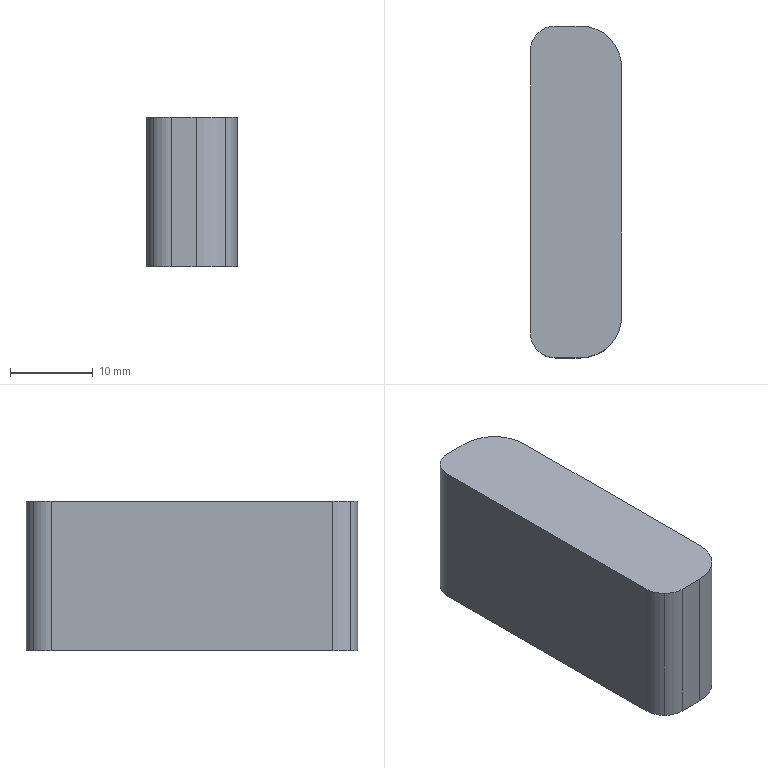Part | STEP file | ASND-0110-6.3aq | 1 solid | 14 faces | box 11 x 40 x 18 mm | volume 7657 mm3 | cylinder 8 | plane 6 | commonest cylinder face diameters 6 x4 10 x4
STEP:
#1=CARTESIAN_POINT('',(0.,0.,0.));
#2=DIRECTION('',(0.,0.,1.));
#3=DIRECTION('',(1.,0.,0.));
#4=AXIS2_PLACEMENT_3D('',#1,#2,#3);
#5=CARTESIAN_POINT('',(-191.546,183.474,-18.));
#6=VERTEX_POINT('',#5);
#7=CARTESIAN_POINT('',(-193.011,187.009,-18.));
#8=VERTEX_POINT('',#7);
#9=CARTESIAN_POINT('',(-196.546,183.474,-18.));
#10=DIRECTION('',(0.,0.,1.));
#11=DIRECTION('',(0.7071,0.7071,0.));
#12=AXIS2_PLACEMENT_3D('',#9,#10,#11);
#13=CIRCLE('',#12,5.);
#14=CARTESIAN_POINT('',(-196.546,183.474,-18.));
#15=DIRECTION('',(0.,0.,1.));
#16=DIRECTION('',(0.7071,0.7071,0.));
#17=AXIS2_PLACEMENT_3D('',#14,#15,#16);
#18=CYLINDRICAL_SURFACE('',#17,5.);
#19=CARTESIAN_POINT('',(0.,0.));
#20=DIRECTION('',(1.,0.));
#21=VECTOR('',#20,1.);
#22=LINE('',#19,#21);
#23=(GEOMETRIC_REPRESENTATION_CONTEXT(2)PARAMETRIC_REPRESENTATION_CONTEXT()REPRESENTATION_CONTEXT('',''));
#24=DEFINITIONAL_REPRESENTATION('',(#22),#23);
#25=PCURVE('',#18,#24);
#26=CARTESIAN_POINT('',(-195.546,183.474,-18.));
#27=DIRECTION('',(0.,0.,1.));
#28=DIRECTION('',(0.7071,0.7071,0.));
#29=AXIS2_PLACEMENT_3D('',#26,#27,#28);
#30=PLANE('',#29);
#31=CARTESIAN_POINT('',(-0.7071,0.7071));
#32=DIRECTION('',(1.,0.));
#33=AXIS2_PLACEMENT_2D('',#31,#32);
#34=CIRCLE('',#33,5.);
#35=(GEOMETRIC_REPRESENTATION_CONTEXT(2)PARAMETRIC_REPRESENTATION_CONTEXT()REPRESENTATION_CONTEXT('',''));
#36=DEFINITIONAL_REPRESENTATION('',(#34),#35);
#37=PCURVE('',#30,#36);
#38=SURFACE_CURVE('',#13,(#25,#37),.PCURVE_S1.);
#39=EDGE_CURVE('',#6,#8,#38,.T.);
#40=ORIENTED_EDGE('',*,*,#39,.T.);
#41=CARTESIAN_POINT('',(-193.011,187.009,0.));
#42=VERTEX_POINT('',#41);
#43=CARTESIAN_POINT('',(-193.011,187.009,-18.));
#44=DIRECTION('',(0.,0.,1.));
#45=VECTOR('',#44,1.);
#46=LINE('',#43,#45);
#47=CARTESIAN_POINT('',(6.283,0.));
#48=DIRECTION('',(0.,1.));
#49=VECTOR('',#48,1.);
#50=LINE('',#47,#49);
#51=(GEOMETRIC_REPRESENTATION_CONTEXT(2)PARAMETRIC_REPRESENTATION_CONTEXT()REPRESENTATION_CONTEXT('',''));
#52=DEFINITIONAL_REPRESENTATION('',(#50),#51);
#53=PCURVE('',#18,#52);
#54=CARTESIAN_POINT('',(-196.546,183.474,-18.));
#55=DIRECTION('',(0.,0.,1.));
#56=DIRECTION('',(0.7071,0.7071,0.));
#57=AXIS2_PLACEMENT_3D('',#54,#55,#56);
#58=CYLINDRICAL_SURFACE('',#57,5.);
#59=CARTESIAN_POINT('',(0.,0.));
#60=DIRECTION('',(0.,1.));
#61=VECTOR('',#60,1.);
#62=LINE('',#59,#61);
#63=(GEOMETRIC_REPRESENTATION_CONTEXT(2)PARAMETRIC_REPRESENTATION_CONTEXT()REPRESENTATION_CONTEXT('',''));
#64=DEFINITIONAL_REPRESENTATION('',(#62),#63);
#65=PCURVE('',#58,#64);
#66=SURFACE_CURVE('',#46,(#53,#65),.PCURVE_S1.);
#67=EDGE_CURVE('',#8,#42,#66,.T.);
#68=ORIENTED_EDGE('',*,*,#67,.T.);
#69=CARTESIAN_POINT('',(-191.546,183.474,0.));
#70=VERTEX_POINT('',#69);
#71=CARTESIAN_POINT('',(-196.546,183.474,0.));
#72=DIRECTION('',(0.,0.,-1.));
#73=DIRECTION('',(0.7071,0.7071,0.));
#74=AXIS2_PLACEMENT_3D('',#71,#72,#73);
#75=CIRCLE('',#74,5.);
#76=CARTESIAN_POINT('',(6.283,18.));
#77=DIRECTION('',(-1.,0.));
#78=VECTOR('',#77,1.);
#79=LINE('',#76,#78);
#80=(GEOMETRIC_REPRESENTATION_CONTEXT(2)PARAMETRIC_REPRESENTATION_CONTEXT()REPRESENTATION_CONTEXT('',''));
#81=DEFINITIONAL_REPRESENTATION('',(#79),#80);
#82=PCURVE('',#18,#81);
#83=CARTESIAN_POINT('',(-195.546,183.474,0.));
#84=DIRECTION('',(0.,0.,1.));
#85=DIRECTION('',(0.7071,0.7071,0.));
#86=AXIS2_PLACEMENT_3D('',#83,#84,#85);
#87=PLANE('',#86);
#88=CARTESIAN_POINT('',(4.293,0.7071));
#89=CARTESIAN_POINT('',(4.293,-7.953));
#90=CARTESIAN_POINT('',(-3.207,-3.623));
#91=CARTESIAN_POINT('',(-10.707,0.7071));
#92=CARTESIAN_POINT('',(-3.207,5.037));
#93=CARTESIAN_POINT('',(4.293,9.367));
#94=CARTESIAN_POINT('',(4.293,0.7071));
#95=(BOUNDED_CURVE()B_SPLINE_CURVE(2,(#88,#89,#90,#91,#92,#93,#94),.UNSPECIFIED.,.T.,.F.)B_SPLINE_CURVE_WITH_KNOTS((1,2,2,2,2,1),(-2.094,0.,2.094,4.189,6.283,8.378),.UNSPECIFIED.)CURVE()GEOMETRIC_REPRESENTATION_ITEM()RATIONAL_B_SPLINE_CURVE((1.,0.5,1.,0.5,1.,0.5,1.))REPRESENTATION_ITEM(''));
#96=(GEOMETRIC_REPRESENTATION_CONTEXT(2)PARAMETRIC_REPRESENTATION_CONTEXT()REPRESENTATION_CONTEXT('',''));
#97=DEFINITIONAL_REPRESENTATION('',(#95),#96);
#98=PCURVE('',#87,#97);
#99=SURFACE_CURVE('',#75,(#82,#98),.PCURVE_S1.);
#100=EDGE_CURVE('',#42,#70,#99,.T.);
#101=ORIENTED_EDGE('',*,*,#100,.T.);
#102=CARTESIAN_POINT('',(-191.546,183.474,-18.));
#103=DIRECTION('',(0.,0.,-1.));
#104=VECTOR('',#103,1.);
#105=LINE('',#102,#104);
#106=CARTESIAN_POINT('',(5.498,0.));
#107=DIRECTION('',(0.,-1.));
#108=VECTOR('',#107,1.);
#109=LINE('',#106,#108);
#110=(GEOMETRIC_REPRESENTATION_CONTEXT(2)PARAMETRIC_REPRESENTATION_CONTEXT()REPRESENTATION_CONTEXT('',''));
#111=DEFINITIONAL_REPRESENTATION('',(#109),#110);
#112=PCURVE('',#18,#111);
#113=CARTESIAN_POINT('',(-191.546,183.474,-18.));
#114=DIRECTION('',(1.,0.,0.));
#115=DIRECTION('',(0.,0.7071,0.7071));
#116=AXIS2_PLACEMENT_3D('',#113,#114,#115);
#117=PLANE('',#116);
#118=CARTESIAN_POINT('',(0.,0.));
#119=DIRECTION('',(-0.7071,-0.7071));
#120=VECTOR('',#119,1.);
#121=LINE('',#118,#120);
#122=(GEOMETRIC_REPRESENTATION_CONTEXT(2)PARAMETRIC_REPRESENTATION_CONTEXT()REPRESENTATION_CONTEXT('',''));
#123=DEFINITIONAL_REPRESENTATION('',(#121),#122);
#124=PCURVE('',#117,#123);
#125=SURFACE_CURVE('',#105,(#112,#124),.PCURVE_S1.);
#126=EDGE_CURVE('',#70,#6,#125,.T.);
#127=ORIENTED_EDGE('',*,*,#126,.T.);
#128=EDGE_LOOP('',(#40,#68,#101,#127));
#129=FACE_BOUND('',#128,.T.);
#130=ADVANCED_FACE('',(#129),#18,.T.);
#131=CARTESIAN_POINT('',(-196.546,148.474,-18.));
#132=VERTEX_POINT('',#131);
#133=CARTESIAN_POINT('',(-193.011,149.938,-18.));
#134=VERTEX_POINT('',#133);
#135=CARTESIAN_POINT('',(-196.546,153.474,-18.));
#136=DIRECTION('',(0.,0.,1.));
#137=DIRECTION('',(0.7071,-0.7071,0.));
#138=AXIS2_PLACEMENT_3D('',#135,#136,#137);
#139=CIRCLE('',#138,5.);
#140=CARTESIAN_POINT('',(-196.546,153.474,-18.));
#141=DIRECTION('',(0.,0.,1.));
#142=DIRECTION('',(0.7071,-0.7071,0.));
#143=AXIS2_PLACEMENT_3D('',#140,#141,#142);
#144=CYLINDRICAL_SURFACE('',#143,5.);
#145=CARTESIAN_POINT('',(0.,0.));
#146=DIRECTION('',(1.,0.));
#147=VECTOR('',#146,1.);
#148=LINE('',#145,#147);
#149=(GEOMETRIC_REPRESENTATION_CONTEXT(2)PARAMETRIC_REPRESENTATION_CONTEXT()REPRESENTATION_CONTEXT('',''));
#150=DEFINITIONAL_REPRESENTATION('',(#148),#149);
#151=PCURVE('',#144,#150);
#152=CARTESIAN_POINT('',(-21.92,-20.506));
#153=DIRECTION('',(0.,-1.));
#154=AXIS2_PLACEMENT_2D('',#152,#153);
#155=CIRCLE('',#154,5.);
#156=(GEOMETRIC_REPRESENTATION_CONTEXT(2)PARAMETRIC_REPRESENTATION_CONTEXT()REPRESENTATION_CONTEXT('',''));
#157=DEFINITIONAL_REPRESENTATION('',(#155),#156);
#158=PCURVE('',#30,#157);
#159=SURFACE_CURVE('',#139,(#151,#158),.PCURVE_S1.);
#160=EDGE_CURVE('',#132,#134,#159,.T.);
#161=ORIENTED_EDGE('',*,*,#160,.T.);
#162=CARTESIAN_POINT('',(-193.011,149.938,0.));
#163=VERTEX_POINT('',#162);
#164=CARTESIAN_POINT('',(-193.011,149.938,-18.));
#165=DIRECTION('',(0.,0.,1.));
#166=VECTOR('',#165,1.);
#167=LINE('',#164,#166);
#168=CARTESIAN_POINT('',(6.283,0.));
#169=DIRECTION('',(0.,1.));
#170=VECTOR('',#169,1.);
#171=LINE('',#168,#170);
#172=(GEOMETRIC_REPRESENTATION_CONTEXT(2)PARAMETRIC_REPRESENTATION_CONTEXT()REPRESENTATION_CONTEXT('',''));
#173=DEFINITIONAL_REPRESENTATION('',(#171),#172);
#174=PCURVE('',#144,#173);
#175=CARTESIAN_POINT('',(-196.546,153.474,-18.));
#176=DIRECTION('',(0.,0.,1.));
#177=DIRECTION('',(0.7071,-0.7071,0.));
#178=AXIS2_PLACEMENT_3D('',#175,#176,#177);
#179=CYLINDRICAL_SURFACE('',#178,5.);
#180=CARTESIAN_POINT('',(0.,0.));
#181=DIRECTION('',(0.,1.));
#182=VECTOR('',#181,1.);
#183=LINE('',#180,#182);
#184=(GEOMETRIC_REPRESENTATION_CONTEXT(2)PARAMETRIC_REPRESENTATION_CONTEXT()REPRESENTATION_CONTEXT('',''));
#185=DEFINITIONAL_REPRESENTATION('',(#183),#184);
#186=PCURVE('',#179,#185);
#187=SURFACE_CURVE('',#167,(#174,#186),.PCURVE_S1.);
#188=EDGE_CURVE('',#134,#163,#187,.T.);
#189=ORIENTED_EDGE('',*,*,#188,.T.);
#190=CARTESIAN_POINT('',(-196.546,148.474,0.));
#191=VERTEX_POINT('',#190);
#192=CARTESIAN_POINT('',(-196.546,153.474,0.));
#193=DIRECTION('',(0.,0.,-1.));
#194=DIRECTION('',(0.7071,-0.7071,0.));
#195=AXIS2_PLACEMENT_3D('',#192,#193,#194);
#196=CIRCLE('',#195,5.);
#197=CARTESIAN_POINT('',(6.283,18.));
#198=DIRECTION('',(-1.,0.));
#199=VECTOR('',#198,1.);
#200=LINE('',#197,#199);
#201=(GEOMETRIC_REPRESENTATION_CONTEXT(2)PARAMETRIC_REPRESENTATION_CONTEXT()REPRESENTATION_CONTEXT('',''));
#202=DEFINITIONAL_REPRESENTATION('',(#200),#201);
#203=PCURVE('',#144,#202);
#204=CARTESIAN_POINT('',(-21.92,-25.506));
#205=CARTESIAN_POINT('',(-30.581,-25.506));
#206=CARTESIAN_POINT('',(-26.25,-18.006));
#207=CARTESIAN_POINT('',(-21.92,-10.506));
#208=CARTESIAN_POINT('',(-17.59,-18.006));
#209=CARTESIAN_POINT('',(-13.26,-25.506));
#210=CARTESIAN_POINT('',(-21.92,-25.506));
#211=(BOUNDED_CURVE()B_SPLINE_CURVE(2,(#204,#205,#206,#207,#208,#209,#210),.UNSPECIFIED.,.T.,.F.)B_SPLINE_CURVE_WITH_KNOTS((1,2,2,2,2,1),(-2.094,0.,2.094,4.189,6.283,8.378),.UNSPECIFIED.)CURVE()GEOMETRIC_REPRESENTATION_ITEM()RATIONAL_B_SPLINE_CURVE((1.,0.5,1.,0.5,1.,0.5,1.))REPRESENTATION_ITEM(''));
#212=(GEOMETRIC_REPRESENTATION_CONTEXT(2)PARAMETRIC_REPRESENTATION_CONTEXT()REPRESENTATION_CONTEXT('',''));
#213=DEFINITIONAL_REPRESENTATION('',(#211),#212);
#214=PCURVE('',#87,#213);
#215=SURFACE_CURVE('',#196,(#203,#214),.PCURVE_S1.);
#216=EDGE_CURVE('',#163,#191,#215,.T.);
#217=ORIENTED_EDGE('',*,*,#216,.T.);
#218=CARTESIAN_POINT('',(-196.546,148.474,-18.));
#219=DIRECTION('',(0.,0.,-1.));
#220=VECTOR('',#219,1.);
#221=LINE('',#218,#220);
#222=CARTESIAN_POINT('',(5.498,0.));
#223=DIRECTION('',(0.,-1.));
#224=VECTOR('',#223,1.);
#225=LINE('',#222,#224);
#226=(GEOMETRIC_REPRESENTATION_CONTEXT(2)PARAMETRIC_REPRESENTATION_CONTEXT()REPRESENTATION_CONTEXT('',''));
#227=DEFINITIONAL_REPRESENTATION('',(#225),#226);
#228=PCURVE('',#144,#227);
#229=CARTESIAN_POINT('',(-195.546,148.474,-18.));
#230=DIRECTION('',(0.,-1.,0.));
#231=DIRECTION('',(0.7071,0.,0.7071));
#232=AXIS2_PLACEMENT_3D('',#229,#230,#231);
#233=PLANE('',#232);
#234=CARTESIAN_POINT('',(-0.7071,0.7071));
#235=DIRECTION('',(-0.7071,-0.7071));
#236=VECTOR('',#235,1.);
#237=LINE('',#234,#236);
#238=(GEOMETRIC_REPRESENTATION_CONTEXT(2)PARAMETRIC_REPRESENTATION_CONTEXT()REPRESENTATION_CONTEXT('',''));
#239=DEFINITIONAL_REPRESENTATION('',(#237),#238);
#240=PCURVE('',#233,#239);
#241=SURFACE_CURVE('',#221,(#228,#240),.PCURVE_S1.);
#242=EDGE_CURVE('',#191,#132,#241,.T.);
#243=ORIENTED_EDGE('',*,*,#242,.T.);
#244=EDGE_LOOP('',(#161,#189,#217,#243));
#245=FACE_BOUND('',#244,.T.);
#246=ADVANCED_FACE('',(#245),#144,.T.);
#247=CARTESIAN_POINT('',(-199.546,148.474,0.));
#248=VERTEX_POINT('',#247);
#249=CARTESIAN_POINT('',(-201.668,149.352,0.));
#250=VERTEX_POINT('',#249);
#251=CARTESIAN_POINT('',(-199.546,151.474,0.));
#252=DIRECTION('',(0.,0.,-1.));
#253=DIRECTION('',(-0.7071,-0.7071,0.));
#254=AXIS2_PLACEMENT_3D('',#251,#252,#253);
#255=CIRCLE('',#254,3.);
#256=CARTESIAN_POINT('',(-199.546,151.474,-18.));
#257=DIRECTION('',(0.,0.,-1.));
#258=DIRECTION('',(-0.7071,-0.7071,0.));
#259=AXIS2_PLACEMENT_3D('',#256,#257,#258);
#260=CYLINDRICAL_SURFACE('',#259,3.);
#261=CARTESIAN_POINT('',(0.,-18.));
#262=DIRECTION('',(1.,0.));
#263=VECTOR('',#262,1.);
#264=LINE('',#261,#263);
#265=(GEOMETRIC_REPRESENTATION_CONTEXT(2)PARAMETRIC_REPRESENTATION_CONTEXT()REPRESENTATION_CONTEXT('',''));
#266=DEFINITIONAL_REPRESENTATION('',(#264),#265);
#267=PCURVE('',#260,#266);
#268=CARTESIAN_POINT('',(-28.456,-19.799));
#269=CARTESIAN_POINT('',(-28.456,-14.603));
#270=CARTESIAN_POINT('',(-23.956,-17.201));
#271=CARTESIAN_POINT('',(-19.456,-19.799));
#272=CARTESIAN_POINT('',(-23.956,-22.397));
#273=CARTESIAN_POINT('',(-28.456,-24.995));
#274=CARTESIAN_POINT('',(-28.456,-19.799));
#275=(BOUNDED_CURVE()B_SPLINE_CURVE(2,(#268,#269,#270,#271,#272,#273,#274),.UNSPECIFIED.,.T.,.F.)B_SPLINE_CURVE_WITH_KNOTS((1,2,2,2,2,1),(-2.094,0.,2.094,4.189,6.283,8.378),.UNSPECIFIED.)CURVE()GEOMETRIC_REPRESENTATION_ITEM()RATIONAL_B_SPLINE_CURVE((1.,0.5,1.,0.5,1.,0.5,1.))REPRESENTATION_ITEM(''));
#276=(GEOMETRIC_REPRESENTATION_CONTEXT(2)PARAMETRIC_REPRESENTATION_CONTEXT()REPRESENTATION_CONTEXT('',''));
#277=DEFINITIONAL_REPRESENTATION('',(#275),#276);
#278=PCURVE('',#87,#277);
#279=SURFACE_CURVE('',#255,(#267,#278),.PCURVE_S1.);
#280=EDGE_CURVE('',#248,#250,#279,.T.);
#281=ORIENTED_EDGE('',*,*,#280,.T.);
#282=CARTESIAN_POINT('',(-201.668,149.352,-18.));
#283=VERTEX_POINT('',#282);
#284=CARTESIAN_POINT('',(-201.668,149.352,-18.));
#285=DIRECTION('',(0.,0.,-1.));
#286=VECTOR('',#285,1.);
#287=LINE('',#284,#286);
#288=CARTESIAN_POINT('',(6.283,0.));
#289=DIRECTION('',(0.,1.));
#290=VECTOR('',#289,1.);
#291=LINE('',#288,#290);
#292=(GEOMETRIC_REPRESENTATION_CONTEXT(2)PARAMETRIC_REPRESENTATION_CONTEXT()REPRESENTATION_CONTEXT('',''));
#293=DEFINITIONAL_REPRESENTATION('',(#291),#292);
#294=PCURVE('',#260,#293);
#295=CARTESIAN_POINT('',(-199.546,151.474,-18.));
#296=DIRECTION('',(0.,0.,-1.));
#297=DIRECTION('',(-0.7071,-0.7071,0.));
#298=AXIS2_PLACEMENT_3D('',#295,#296,#297);
#299=CYLINDRICAL_SURFACE('',#298,3.);
#300=CARTESIAN_POINT('',(0.,0.));
#301=DIRECTION('',(0.,1.));
#302=VECTOR('',#301,1.);
#303=LINE('',#300,#302);
#304=(GEOMETRIC_REPRESENTATION_CONTEXT(2)PARAMETRIC_REPRESENTATION_CONTEXT()REPRESENTATION_CONTEXT('',''));
#305=DEFINITIONAL_REPRESENTATION('',(#303),#304);
#306=PCURVE('',#299,#305);
#307=SURFACE_CURVE('',#287,(#294,#306),.PCURVE_S1.);
#308=EDGE_CURVE('',#250,#283,#307,.T.);
#309=ORIENTED_EDGE('',*,*,#308,.T.);
#310=CARTESIAN_POINT('',(-199.546,148.474,-18.));
#311=VERTEX_POINT('',#310);
#312=CARTESIAN_POINT('',(-199.546,151.474,-18.));
#313=DIRECTION('',(0.,0.,1.));
#314=DIRECTION('',(-0.7071,-0.7071,0.));
#315=AXIS2_PLACEMENT_3D('',#312,#313,#314);
#316=CIRCLE('',#315,3.);
#317=CARTESIAN_POINT('',(6.283,0.));
#318=DIRECTION('',(-1.,0.));
#319=VECTOR('',#318,1.);
#320=LINE('',#317,#319);
#321=(GEOMETRIC_REPRESENTATION_CONTEXT(2)PARAMETRIC_REPRESENTATION_CONTEXT()REPRESENTATION_CONTEXT('',''));
#322=DEFINITIONAL_REPRESENTATION('',(#320),#321);
#323=PCURVE('',#260,#322);
#324=CARTESIAN_POINT('',(-25.456,-19.799));
#325=DIRECTION('',(-1.,0.));
#326=AXIS2_PLACEMENT_2D('',#324,#325);
#327=CIRCLE('',#326,3.);
#328=(GEOMETRIC_REPRESENTATION_CONTEXT(2)PARAMETRIC_REPRESENTATION_CONTEXT()REPRESENTATION_CONTEXT('',''));
#329=DEFINITIONAL_REPRESENTATION('',(#327),#328);
#330=PCURVE('',#30,#329);
#331=SURFACE_CURVE('',#316,(#323,#330),.PCURVE_S1.);
#332=EDGE_CURVE('',#283,#311,#331,.T.);
#333=ORIENTED_EDGE('',*,*,#332,.T.);
#334=CARTESIAN_POINT('',(-199.546,148.474,-18.));
#335=DIRECTION('',(0.,0.,1.));
#336=VECTOR('',#335,1.);
#337=LINE('',#334,#336);
#338=CARTESIAN_POINT('',(5.498,0.));
#339=DIRECTION('',(0.,-1.));
#340=VECTOR('',#339,1.);
#341=LINE('',#338,#340);
#342=(GEOMETRIC_REPRESENTATION_CONTEXT(2)PARAMETRIC_REPRESENTATION_CONTEXT()REPRESENTATION_CONTEXT('',''));
#343=DEFINITIONAL_REPRESENTATION('',(#341),#342);
#344=PCURVE('',#260,#343);
#345=CARTESIAN_POINT('',(-2.828,2.828));
#346=DIRECTION('',(0.7071,0.7071));
#347=VECTOR('',#346,1.);
#348=LINE('',#345,#347);
#349=(GEOMETRIC_REPRESENTATION_CONTEXT(2)PARAMETRIC_REPRESENTATION_CONTEXT()REPRESENTATION_CONTEXT('',''));
#350=DEFINITIONAL_REPRESENTATION('',(#348),#349);
#351=PCURVE('',#233,#350);
#352=SURFACE_CURVE('',#337,(#344,#351),.PCURVE_S1.);
#353=EDGE_CURVE('',#311,#248,#352,.T.);
#354=ORIENTED_EDGE('',*,*,#353,.T.);
#355=EDGE_LOOP('',(#281,#309,#333,#354));
#356=FACE_BOUND('',#355,.T.);
#357=ADVANCED_FACE('',(#356),#260,.T.);
#358=CARTESIAN_POINT('',(-202.546,185.474,0.));
#359=VERTEX_POINT('',#358);
#360=CARTESIAN_POINT('',(-201.668,187.595,0.));
#361=VERTEX_POINT('',#360);
#362=CARTESIAN_POINT('',(-199.546,185.474,0.));
#363=DIRECTION('',(0.,0.,-1.));
#364=DIRECTION('',(-0.7071,0.7071,0.));
#365=AXIS2_PLACEMENT_3D('',#362,#363,#364);
#366=CIRCLE('',#365,3.);
#367=CARTESIAN_POINT('',(-199.546,185.474,-18.));
#368=DIRECTION('',(0.,0.,-1.));
#369=DIRECTION('',(-0.7071,0.7071,0.));
#370=AXIS2_PLACEMENT_3D('',#367,#368,#369);
#371=CYLINDRICAL_SURFACE('',#370,3.);
#372=CARTESIAN_POINT('',(0.,-18.));
#373=DIRECTION('',(1.,0.));
#374=VECTOR('',#373,1.);
#375=LINE('',#372,#374);
#376=(GEOMETRIC_REPRESENTATION_CONTEXT(2)PARAMETRIC_REPRESENTATION_CONTEXT()REPRESENTATION_CONTEXT('',''));
#377=DEFINITIONAL_REPRESENTATION('',(#375),#376);
#378=PCURVE('',#371,#377);
#379=CARTESIAN_POINT('',(-1.414,7.243));
#380=CARTESIAN_POINT('',(3.782,7.243));
#381=CARTESIAN_POINT('',(1.184,2.743));
#382=CARTESIAN_POINT('',(-1.414,-1.757));
#383=CARTESIAN_POINT('',(-4.012,2.743));
#384=CARTESIAN_POINT('',(-6.61,7.243));
#385=CARTESIAN_POINT('',(-1.414,7.243));
#386=(BOUNDED_CURVE()B_SPLINE_CURVE(2,(#379,#380,#381,#382,#383,#384,#385),.UNSPECIFIED.,.T.,.F.)B_SPLINE_CURVE_WITH_KNOTS((1,2,2,2,2,1),(-2.094,0.,2.094,4.189,6.283,8.378),.UNSPECIFIED.)CURVE()GEOMETRIC_REPRESENTATION_ITEM()RATIONAL_B_SPLINE_CURVE((1.,0.5,1.,0.5,1.,0.5,1.))REPRESENTATION_ITEM(''));
#387=(GEOMETRIC_REPRESENTATION_CONTEXT(2)PARAMETRIC_REPRESENTATION_CONTEXT()REPRESENTATION_CONTEXT('',''));
#388=DEFINITIONAL_REPRESENTATION('',(#386),#387);
#389=PCURVE('',#87,#388);
#390=SURFACE_CURVE('',#366,(#378,#389),.PCURVE_S1.);
#391=EDGE_CURVE('',#359,#361,#390,.T.);
#392=ORIENTED_EDGE('',*,*,#391,.T.);
#393=CARTESIAN_POINT('',(-201.668,187.595,-18.));
#394=VERTEX_POINT('',#393);
#395=CARTESIAN_POINT('',(-201.668,187.595,-18.));
#396=DIRECTION('',(0.,0.,-1.));
#397=VECTOR('',#396,1.);
#398=LINE('',#395,#397);
#399=CARTESIAN_POINT('',(6.283,0.));
#400=DIRECTION('',(0.,1.));
#401=VECTOR('',#400,1.);
#402=LINE('',#399,#401);
#403=(GEOMETRIC_REPRESENTATION_CONTEXT(2)PARAMETRIC_REPRESENTATION_CONTEXT()REPRESENTATION_CONTEXT('',''));
#404=DEFINITIONAL_REPRESENTATION('',(#402),#403);
#405=PCURVE('',#371,#404);
#406=CARTESIAN_POINT('',(-199.546,185.474,-18.));
#407=DIRECTION('',(0.,0.,-1.));
#408=DIRECTION('',(-0.7071,0.7071,0.));
#409=AXIS2_PLACEMENT_3D('',#406,#407,#408);
#410=CYLINDRICAL_SURFACE('',#409,3.);
#411=CARTESIAN_POINT('',(0.,0.));
#412=DIRECTION('',(0.,1.));
#413=VECTOR('',#412,1.);
#414=LINE('',#411,#413);
#415=(GEOMETRIC_REPRESENTATION_CONTEXT(2)PARAMETRIC_REPRESENTATION_CONTEXT()REPRESENTATION_CONTEXT('',''));
#416=DEFINITIONAL_REPRESENTATION('',(#414),#415);
#417=PCURVE('',#410,#416);
#418=SURFACE_CURVE('',#398,(#405,#417),.PCURVE_S1.);
#419=EDGE_CURVE('',#361,#394,#418,.T.);
#420=ORIENTED_EDGE('',*,*,#419,.T.);
#421=CARTESIAN_POINT('',(-202.546,185.474,-18.));
#422=VERTEX_POINT('',#421);
#423=CARTESIAN_POINT('',(-199.546,185.474,-18.));
#424=DIRECTION('',(0.,0.,1.));
#425=DIRECTION('',(-0.7071,0.7071,0.));
#426=AXIS2_PLACEMENT_3D('',#423,#424,#425);
#427=CIRCLE('',#426,3.);
#428=CARTESIAN_POINT('',(6.283,0.));
#429=DIRECTION('',(-1.,0.));
#430=VECTOR('',#429,1.);
#431=LINE('',#428,#430);
#432=(GEOMETRIC_REPRESENTATION_CONTEXT(2)PARAMETRIC_REPRESENTATION_CONTEXT()REPRESENTATION_CONTEXT('',''));
#433=DEFINITIONAL_REPRESENTATION('',(#431),#432);
#434=PCURVE('',#371,#433);
#435=CARTESIAN_POINT('',(-1.414,4.243));
#436=DIRECTION('',(0.,1.));
#437=AXIS2_PLACEMENT_2D('',#435,#436);
#438=CIRCLE('',#437,3.);
#439=(GEOMETRIC_REPRESENTATION_CONTEXT(2)PARAMETRIC_REPRESENTATION_CONTEXT()REPRESENTATION_CONTEXT('',''));
#440=DEFINITIONAL_REPRESENTATION('',(#438),#439);
#441=PCURVE('',#30,#440);
#442=SURFACE_CURVE('',#427,(#434,#441),.PCURVE_S1.);
#443=EDGE_CURVE('',#394,#422,#442,.T.);
#444=ORIENTED_EDGE('',*,*,#443,.T.);
#445=CARTESIAN_POINT('',(-202.546,185.474,-18.));
#446=DIRECTION('',(0.,0.,1.));
#447=VECTOR('',#446,1.);
#448=LINE('',#445,#447);
#449=CARTESIAN_POINT('',(5.498,0.));
#450=DIRECTION('',(0.,-1.));
#451=VECTOR('',#450,1.);
#452=LINE('',#449,#451);
#453=(GEOMETRIC_REPRESENTATION_CONTEXT(2)PARAMETRIC_REPRESENTATION_CONTEXT()REPRESENTATION_CONTEXT('',''));
#454=DEFINITIONAL_REPRESENTATION('',(#452),#453);
#455=PCURVE('',#371,#454);
#456=CARTESIAN_POINT('',(-202.546,185.474,-18.));
#457=DIRECTION('',(-1.,0.,0.));
#458=DIRECTION('',(0.,0.7071,0.7071));
#459=AXIS2_PLACEMENT_3D('',#456,#457,#458);
#460=PLANE('',#459);
#461=CARTESIAN_POINT('',(0.,0.));
#462=DIRECTION('',(0.7071,-0.7071));
#463=VECTOR('',#462,1.);
#464=LINE('',#461,#463);
#465=(GEOMETRIC_REPRESENTATION_CONTEXT(2)PARAMETRIC_REPRESENTATION_CONTEXT()REPRESENTATION_CONTEXT('',''));
#466=DEFINITIONAL_REPRESENTATION('',(#464),#465);
#467=PCURVE('',#460,#466);
#468=SURFACE_CURVE('',#448,(#455,#467),.PCURVE_S1.);
#469=EDGE_CURVE('',#422,#359,#468,.T.);
#470=ORIENTED_EDGE('',*,*,#469,.T.);
#471=EDGE_LOOP('',(#392,#420,#444,#470));
#472=FACE_BOUND('',#471,.T.);
#473=ADVANCED_FACE('',(#472),#371,.T.);
#474=ORIENTED_EDGE('',*,*,#419,.F.);
#475=CARTESIAN_POINT('',(-199.546,188.474,0.));
#476=VERTEX_POINT('',#475);
#477=CARTESIAN_POINT('',(-199.546,185.474,0.));
#478=DIRECTION('',(0.,0.,-1.));
#479=DIRECTION('',(-0.7071,0.7071,0.));
#480=AXIS2_PLACEMENT_3D('',#477,#478,#479);
#481=CIRCLE('',#480,3.);
#482=CARTESIAN_POINT('',(0.,-18.));
#483=DIRECTION('',(1.,0.));
#484=VECTOR('',#483,1.);
#485=LINE('',#482,#484);
#486=(GEOMETRIC_REPRESENTATION_CONTEXT(2)PARAMETRIC_REPRESENTATION_CONTEXT()REPRESENTATION_CONTEXT('',''));
#487=DEFINITIONAL_REPRESENTATION('',(#485),#486);
#488=PCURVE('',#410,#487);
#489=CARTESIAN_POINT('',(-1.414,7.243));
#490=CARTESIAN_POINT('',(3.782,7.243));
#491=CARTESIAN_POINT('',(1.184,2.743));
#492=CARTESIAN_POINT('',(-1.414,-1.757));
#493=CARTESIAN_POINT('',(-4.012,2.743));
#494=CARTESIAN_POINT('',(-6.61,7.243));
#495=CARTESIAN_POINT('',(-1.414,7.243));
#496=(BOUNDED_CURVE()B_SPLINE_CURVE(2,(#489,#490,#491,#492,#493,#494,#495),.UNSPECIFIED.,.T.,.F.)B_SPLINE_CURVE_WITH_KNOTS((1,2,2,2,2,1),(-2.094,0.,2.094,4.189,6.283,8.378),.UNSPECIFIED.)CURVE()GEOMETRIC_REPRESENTATION_ITEM()RATIONAL_B_SPLINE_CURVE((1.,0.5,1.,0.5,1.,0.5,1.))REPRESENTATION_ITEM(''));
#497=(GEOMETRIC_REPRESENTATION_CONTEXT(2)PARAMETRIC_REPRESENTATION_CONTEXT()REPRESENTATION_CONTEXT('',''));
#498=DEFINITIONAL_REPRESENTATION('',(#496),#497);
#499=PCURVE('',#87,#498);
#500=SURFACE_CURVE('',#481,(#488,#499),.PCURVE_S1.);
#501=EDGE_CURVE('',#361,#476,#500,.T.);
#502=ORIENTED_EDGE('',*,*,#501,.T.);
#503=CARTESIAN_POINT('',(-199.546,188.474,-18.));
#504=VERTEX_POINT('',#503);
#505=CARTESIAN_POINT('',(-199.546,188.474,-18.));
#506=DIRECTION('',(0.,0.,-1.));
#507=VECTOR('',#506,1.);
#508=LINE('',#505,#507);
#509=CARTESIAN_POINT('',(0.7854,0.));
#510=DIRECTION('',(0.,1.));
#511=VECTOR('',#510,1.);
#512=LINE('',#509,#511);
#513=(GEOMETRIC_REPRESENTATION_CONTEXT(2)PARAMETRIC_REPRESENTATION_CONTEXT()REPRESENTATION_CONTEXT('',''));
#514=DEFINITIONAL_REPRESENTATION('',(#512),#513);
#515=PCURVE('',#410,#514);
#516=CARTESIAN_POINT('',(-197.546,188.474,-18.));
#517=DIRECTION('',(0.,1.,0.));
#518=DIRECTION('',(0.7071,0.,0.7071));
#519=AXIS2_PLACEMENT_3D('',#516,#517,#518);
#520=PLANE('',#519);
#521=CARTESIAN_POINT('',(-1.414,-1.414));
#522=DIRECTION('',(-0.7071,0.7071));
#523=VECTOR('',#522,1.);
#524=LINE('',#521,#523);
#525=(GEOMETRIC_REPRESENTATION_CONTEXT(2)PARAMETRIC_REPRESENTATION_CONTEXT()REPRESENTATION_CONTEXT('',''));
#526=DEFINITIONAL_REPRESENTATION('',(#524),#525);
#527=PCURVE('',#520,#526);
#528=SURFACE_CURVE('',#508,(#515,#527),.PCURVE_S1.);
#529=EDGE_CURVE('',#476,#504,#528,.T.);
#530=ORIENTED_EDGE('',*,*,#529,.T.);
#531=CARTESIAN_POINT('',(-199.546,185.474,-18.));
#532=DIRECTION('',(0.,0.,1.));
#533=DIRECTION('',(-0.7071,0.7071,0.));
#534=AXIS2_PLACEMENT_3D('',#531,#532,#533);
#535=CIRCLE('',#534,3.);
#536=CARTESIAN_POINT('',(6.283,0.));
#537=DIRECTION('',(-1.,0.));
#538=VECTOR('',#537,1.);
#539=LINE('',#536,#538);
#540=(GEOMETRIC_REPRESENTATION_CONTEXT(2)PARAMETRIC_REPRESENTATION_CONTEXT()REPRESENTATION_CONTEXT('',''));
#541=DEFINITIONAL_REPRESENTATION('',(#539),#540);
#542=PCURVE('',#410,#541);
#543=CARTESIAN_POINT('',(-1.414,4.243));
#544=DIRECTION('',(0.,1.));
#545=AXIS2_PLACEMENT_2D('',#543,#544);
#546=CIRCLE('',#545,3.);
#547=(GEOMETRIC_REPRESENTATION_CONTEXT(2)PARAMETRIC_REPRESENTATION_CONTEXT()REPRESENTATION_CONTEXT('',''));
#548=DEFINITIONAL_REPRESENTATION('',(#546),#547);
#549=PCURVE('',#30,#548);
#550=SURFACE_CURVE('',#535,(#542,#549),.PCURVE_S1.);
#551=EDGE_CURVE('',#504,#394,#550,.T.);
#552=ORIENTED_EDGE('',*,*,#551,.T.);
#553=EDGE_LOOP('',(#474,#502,#530,#552));
#554=FACE_BOUND('',#553,.T.);
#555=ADVANCED_FACE('',(#554),#410,.T.);
#556=ORIENTED_EDGE('',*,*,#529,.F.);
#557=CARTESIAN_POINT('',(-196.546,188.474,0.));
#558=VERTEX_POINT('',#557);
#559=CARTESIAN_POINT('',(-195.546,188.474,0.));
#560=DIRECTION('',(-1.,0.,0.));
#561=VECTOR('',#560,1.);
#562=LINE('',#559,#561);
#563=CARTESIAN_POINT('',(14.142,-11.314));
#564=DIRECTION('',(-0.7071,-0.7071));
#565=VECTOR('',#564,1.);
#566=LINE('',#563,#565);
#567=(GEOMETRIC_REPRESENTATION_CONTEXT(2)PARAMETRIC_REPRESENTATION_CONTEXT()REPRESENTATION_CONTEXT('',''));
#568=DEFINITIONAL_REPRESENTATION('',(#566),#567);
#569=PCURVE('',#520,#568);
#570=CARTESIAN_POINT('',(3.536,3.536));
#571=DIRECTION('',(-0.7071,0.7071));
#572=VECTOR('',#571,1.);
#573=LINE('',#570,#572);
#574=(GEOMETRIC_REPRESENTATION_CONTEXT(2)PARAMETRIC_REPRESENTATION_CONTEXT()REPRESENTATION_CONTEXT('',''));
#575=DEFINITIONAL_REPRESENTATION('',(#573),#574);
#576=PCURVE('',#87,#575);
#577=SURFACE_CURVE('',#562,(#569,#576),.PCURVE_S1.);
#578=EDGE_CURVE('',#558,#476,#577,.T.);
#579=ORIENTED_EDGE('',*,*,#578,.F.);
#580=CARTESIAN_POINT('',(-196.546,188.474,-18.));
#581=VERTEX_POINT('',#580);
#582=CARTESIAN_POINT('',(-196.546,188.474,-18.));
#583=DIRECTION('',(0.,0.,1.));
#584=VECTOR('',#583,1.);
#585=LINE('',#582,#584);
#586=CARTESIAN_POINT('',(0.7071,0.7071));
#587=DIRECTION('',(0.7071,-0.7071));
#588=VECTOR('',#587,1.);
#589=LINE('',#586,#588);
#590=(GEOMETRIC_REPRESENTATION_CONTEXT(2)PARAMETRIC_REPRESENTATION_CONTEXT()REPRESENTATION_CONTEXT('',''));
#591=DEFINITIONAL_REPRESENTATION('',(#589),#590);
#592=PCURVE('',#520,#591);
#593=CARTESIAN_POINT('',(0.7854,0.));
#594=DIRECTION('',(0.,1.));
#595=VECTOR('',#594,1.);
#596=LINE('',#593,#595);
#597=(GEOMETRIC_REPRESENTATION_CONTEXT(2)PARAMETRIC_REPRESENTATION_CONTEXT()REPRESENTATION_CONTEXT('',''));
#598=DEFINITIONAL_REPRESENTATION('',(#596),#597);
#599=PCURVE('',#58,#598);
#600=SURFACE_CURVE('',#585,(#592,#599),.PCURVE_S1.);
#601=EDGE_CURVE('',#581,#558,#600,.T.);
#602=ORIENTED_EDGE('',*,*,#601,.F.);
#603=CARTESIAN_POINT('',(-195.546,188.474,-18.));
#604=DIRECTION('',(-1.,0.,0.));
#605=VECTOR('',#604,1.);
#606=LINE('',#603,#605);
#607=CARTESIAN_POINT('',(1.414,1.414));
#608=DIRECTION('',(-0.7071,-0.7071));
#609=VECTOR('',#608,1.);
#610=LINE('',#607,#609);
#611=(GEOMETRIC_REPRESENTATION_CONTEXT(2)PARAMETRIC_REPRESENTATION_CONTEXT()REPRESENTATION_CONTEXT('',''));
#612=DEFINITIONAL_REPRESENTATION('',(#610),#611);
#613=PCURVE('',#520,#612);
#614=CARTESIAN_POINT('',(3.536,3.536));
#615=DIRECTION('',(-0.7071,0.7071));
#616=VECTOR('',#615,1.);
#617=LINE('',#614,#616);
#618=(GEOMETRIC_REPRESENTATION_CONTEXT(2)PARAMETRIC_REPRESENTATION_CONTEXT()REPRESENTATION_CONTEXT('',''));
#619=DEFINITIONAL_REPRESENTATION('',(#617),#618);
#620=PCURVE('',#30,#619);
#621=SURFACE_CURVE('',#606,(#613,#620),.PCURVE_S1.);
#622=EDGE_CURVE('',#581,#504,#621,.T.);
#623=ORIENTED_EDGE('',*,*,#622,.T.);
#624=EDGE_LOOP('',(#556,#579,#602,#623));
#625=FACE_BOUND('',#624,.T.);
#626=ADVANCED_FACE('',(#625),#520,.T.);
#627=ORIENTED_EDGE('',*,*,#391,.F.);
#628=CARTESIAN_POINT('',(-202.546,151.474,0.));
#629=VERTEX_POINT('',#628);
#630=CARTESIAN_POINT('',(-202.546,185.474,0.));
#631=DIRECTION('',(0.,-1.,0.));
#632=VECTOR('',#631,1.);
#633=LINE('',#630,#632);
#634=CARTESIAN_POINT('',(-3.536,6.364));
#635=DIRECTION('',(-0.7071,-0.7071));
#636=VECTOR('',#635,1.);
#637=LINE('',#634,#636);
#638=(GEOMETRIC_REPRESENTATION_CONTEXT(2)PARAMETRIC_REPRESENTATION_CONTEXT()REPRESENTATION_CONTEXT('',''));
#639=DEFINITIONAL_REPRESENTATION('',(#637),#638);
#640=PCURVE('',#87,#639);
#641=CARTESIAN_POINT('',(12.728,-12.728));
#642=DIRECTION('',(-0.7071,-0.7071));
#643=VECTOR('',#642,1.);
#644=LINE('',#641,#643);
#645=(GEOMETRIC_REPRESENTATION_CONTEXT(2)PARAMETRIC_REPRESENTATION_CONTEXT()REPRESENTATION_CONTEXT('',''));
#646=DEFINITIONAL_REPRESENTATION('',(#644),#645);
#647=PCURVE('',#460,#646);
#648=SURFACE_CURVE('',#633,(#640,#647),.PCURVE_S1.);
#649=EDGE_CURVE('',#359,#629,#648,.T.);
#650=ORIENTED_EDGE('',*,*,#649,.T.);
#651=CARTESIAN_POINT('',(-199.546,151.474,0.));
#652=DIRECTION('',(0.,0.,-1.));
#653=DIRECTION('',(-0.7071,-0.7071,0.));
#654=AXIS2_PLACEMENT_3D('',#651,#652,#653);
#655=CIRCLE('',#654,3.);
#656=CARTESIAN_POINT('',(-28.456,-19.799));
#657=CARTESIAN_POINT('',(-28.456,-14.603));
#658=CARTESIAN_POINT('',(-23.956,-17.201));
#659=CARTESIAN_POINT('',(-19.456,-19.799));
#660=CARTESIAN_POINT('',(-23.956,-22.397));
#661=CARTESIAN_POINT('',(-28.456,-24.995));
#662=CARTESIAN_POINT('',(-28.456,-19.799));
#663=(BOUNDED_CURVE()B_SPLINE_CURVE(2,(#656,#657,#658,#659,#660,#661,#662),.UNSPECIFIED.,.T.,.F.)B_SPLINE_CURVE_WITH_KNOTS((1,2,2,2,2,1),(-2.094,0.,2.094,4.189,6.283,8.378),.UNSPECIFIED.)CURVE()GEOMETRIC_REPRESENTATION_ITEM()RATIONAL_B_SPLINE_CURVE((1.,0.5,1.,0.5,1.,0.5,1.))REPRESENTATION_ITEM(''));
#664=(GEOMETRIC_REPRESENTATION_CONTEXT(2)PARAMETRIC_REPRESENTATION_CONTEXT()REPRESENTATION_CONTEXT('',''));
#665=DEFINITIONAL_REPRESENTATION('',(#663),#664);
#666=PCURVE('',#87,#665);
#667=CARTESIAN_POINT('',(0.,-18.));
#668=DIRECTION('',(1.,0.));
#669=VECTOR('',#668,1.);
#670=LINE('',#667,#669);
#671=(GEOMETRIC_REPRESENTATION_CONTEXT(2)PARAMETRIC_REPRESENTATION_CONTEXT()REPRESENTATION_CONTEXT('',''));
#672=DEFINITIONAL_REPRESENTATION('',(#670),#671);
#673=PCURVE('',#299,#672);
#674=SURFACE_CURVE('',#655,(#666,#673),.PCURVE_S1.);
#675=EDGE_CURVE('',#250,#629,#674,.T.);
#676=ORIENTED_EDGE('',*,*,#675,.F.);
#677=ORIENTED_EDGE('',*,*,#280,.F.);
#678=CARTESIAN_POINT('',(-197.546,148.474,0.));
#679=DIRECTION('',(1.,0.,0.));
#680=VECTOR('',#679,1.);
#681=LINE('',#678,#680);
#682=CARTESIAN_POINT('',(-26.163,-23.335));
#683=DIRECTION('',(0.7071,-0.7071));
#684=VECTOR('',#683,1.);
#685=LINE('',#682,#684);
#686=(GEOMETRIC_REPRESENTATION_CONTEXT(2)PARAMETRIC_REPRESENTATION_CONTEXT()REPRESENTATION_CONTEXT('',''));
#687=DEFINITIONAL_REPRESENTATION('',(#685),#686);
#688=PCURVE('',#87,#687);
#689=CARTESIAN_POINT('',(11.314,14.142));
#690=DIRECTION('',(0.7071,-0.7071));
#691=VECTOR('',#690,1.);
#692=LINE('',#689,#691);
#693=(GEOMETRIC_REPRESENTATION_CONTEXT(2)PARAMETRIC_REPRESENTATION_CONTEXT()REPRESENTATION_CONTEXT('',''));
#694=DEFINITIONAL_REPRESENTATION('',(#692),#693);
#695=PCURVE('',#233,#694);
#696=SURFACE_CURVE('',#681,(#688,#695),.PCURVE_S1.);
#697=EDGE_CURVE('',#248,#191,#696,.T.);
#698=ORIENTED_EDGE('',*,*,#697,.T.);
#699=ORIENTED_EDGE('',*,*,#216,.F.);
#700=CARTESIAN_POINT('',(-191.546,153.474,0.));
#701=VERTEX_POINT('',#700);
#702=CARTESIAN_POINT('',(-196.546,153.474,0.));
#703=DIRECTION('',(0.,0.,-1.));
#704=DIRECTION('',(0.7071,-0.7071,0.));
#705=AXIS2_PLACEMENT_3D('',#702,#703,#704);
#706=CIRCLE('',#705,5.);
#707=CARTESIAN_POINT('',(-21.92,-25.506));
#708=CARTESIAN_POINT('',(-30.581,-25.506));
#709=CARTESIAN_POINT('',(-26.25,-18.006));
#710=CARTESIAN_POINT('',(-21.92,-10.506));
#711=CARTESIAN_POINT('',(-17.59,-18.006));
#712=CARTESIAN_POINT('',(-13.26,-25.506));
#713=CARTESIAN_POINT('',(-21.92,-25.506));
#714=(BOUNDED_CURVE()B_SPLINE_CURVE(2,(#707,#708,#709,#710,#711,#712,#713),.UNSPECIFIED.,.T.,.F.)B_SPLINE_CURVE_WITH_KNOTS((1,2,2,2,2,1),(-2.094,0.,2.094,4.189,6.283,8.378),.UNSPECIFIED.)CURVE()GEOMETRIC_REPRESENTATION_ITEM()RATIONAL_B_SPLINE_CURVE((1.,0.5,1.,0.5,1.,0.5,1.))REPRESENTATION_ITEM(''));
#715=(GEOMETRIC_REPRESENTATION_CONTEXT(2)PARAMETRIC_REPRESENTATION_CONTEXT()REPRESENTATION_CONTEXT('',''));
#716=DEFINITIONAL_REPRESENTATION('',(#714),#715);
#717=PCURVE('',#87,#716);
#718=CARTESIAN_POINT('',(6.283,18.));
#719=DIRECTION('',(-1.,0.));
#720=VECTOR('',#719,1.);
#721=LINE('',#718,#720);
#722=(GEOMETRIC_REPRESENTATION_CONTEXT(2)PARAMETRIC_REPRESENTATION_CONTEXT()REPRESENTATION_CONTEXT('',''));
#723=DEFINITIONAL_REPRESENTATION('',(#721),#722);
#724=PCURVE('',#179,#723);
#725=SURFACE_CURVE('',#706,(#717,#724),.PCURVE_S1.);
#726=EDGE_CURVE('',#701,#163,#725,.T.);
#727=ORIENTED_EDGE('',*,*,#726,.F.);
#728=CARTESIAN_POINT('',(-191.546,133.474,0.));
#729=DIRECTION('',(0.,1.,0.));
#730=VECTOR('',#729,1.);
#731=LINE('',#728,#730);
#732=CARTESIAN_POINT('',(-32.527,-38.184));
#733=DIRECTION('',(0.7071,0.7071));
#734=VECTOR('',#733,1.);
#735=LINE('',#732,#734);
#736=(GEOMETRIC_REPRESENTATION_CONTEXT(2)PARAMETRIC_REPRESENTATION_CONTEXT()REPRESENTATION_CONTEXT('',''));
#737=DEFINITIONAL_REPRESENTATION('',(#735),#736);
#738=PCURVE('',#87,#737);
#739=CARTESIAN_POINT('',(-22.627,48.083));
#740=DIRECTION('',(0.7071,-0.7071));
#741=VECTOR('',#740,1.);
#742=LINE('',#739,#741);
#743=(GEOMETRIC_REPRESENTATION_CONTEXT(2)PARAMETRIC_REPRESENTATION_CONTEXT()REPRESENTATION_CONTEXT('',''));
#744=DEFINITIONAL_REPRESENTATION('',(#742),#743);
#745=PCURVE('',#117,#744);
#746=SURFACE_CURVE('',#731,(#738,#745),.PCURVE_S1.);
#747=EDGE_CURVE('',#701,#70,#746,.T.);
#748=ORIENTED_EDGE('',*,*,#747,.T.);
#749=ORIENTED_EDGE('',*,*,#100,.F.);
#750=CARTESIAN_POINT('',(-196.546,183.474,0.));
#751=DIRECTION('',(0.,0.,-1.));
#752=DIRECTION('',(0.7071,0.7071,0.));
#753=AXIS2_PLACEMENT_3D('',#750,#751,#752);
#754=CIRCLE('',#753,5.);
#755=CARTESIAN_POINT('',(4.293,0.7071));
#756=CARTESIAN_POINT('',(4.293,-7.953));
#757=CARTESIAN_POINT('',(-3.207,-3.623));
#758=CARTESIAN_POINT('',(-10.707,0.7071));
#759=CARTESIAN_POINT('',(-3.207,5.037));
#760=CARTESIAN_POINT('',(4.293,9.367));
#761=CARTESIAN_POINT('',(4.293,0.7071));
#762=(BOUNDED_CURVE()B_SPLINE_CURVE(2,(#755,#756,#757,#758,#759,#760,#761),.UNSPECIFIED.,.T.,.F.)B_SPLINE_CURVE_WITH_KNOTS((1,2,2,2,2,1),(-2.094,0.,2.094,4.189,6.283,8.378),.UNSPECIFIED.)CURVE()GEOMETRIC_REPRESENTATION_ITEM()RATIONAL_B_SPLINE_CURVE((1.,0.5,1.,0.5,1.,0.5,1.))REPRESENTATION_ITEM(''));
#763=(GEOMETRIC_REPRESENTATION_CONTEXT(2)PARAMETRIC_REPRESENTATION_CONTEXT()REPRESENTATION_CONTEXT('',''));
#764=DEFINITIONAL_REPRESENTATION('',(#762),#763);
#765=PCURVE('',#87,#764);
#766=CARTESIAN_POINT('',(6.283,18.));
#767=DIRECTION('',(-1.,0.));
#768=VECTOR('',#767,1.);
#769=LINE('',#766,#768);
#770=(GEOMETRIC_REPRESENTATION_CONTEXT(2)PARAMETRIC_REPRESENTATION_CONTEXT()REPRESENTATION_CONTEXT('',''));
#771=DEFINITIONAL_REPRESENTATION('',(#769),#770);
#772=PCURVE('',#58,#771);
#773=SURFACE_CURVE('',#754,(#765,#772),.PCURVE_S1.);
#774=EDGE_CURVE('',#558,#42,#773,.T.);
#775=ORIENTED_EDGE('',*,*,#774,.F.);
#776=ORIENTED_EDGE('',*,*,#578,.T.);
#777=ORIENTED_EDGE('',*,*,#501,.F.);
#778=EDGE_LOOP('',(#627,#650,#676,#677,#698,#699,#727,#748,#749,#775,#776,#777));
#779=FACE_BOUND('',#778,.T.);
#780=ADVANCED_FACE('',(#779),#87,.T.);
#781=ORIENTED_EDGE('',*,*,#308,.F.);
#782=ORIENTED_EDGE('',*,*,#675,.T.);
#783=CARTESIAN_POINT('',(-202.546,151.474,-18.));
#784=VERTEX_POINT('',#783);
#785=CARTESIAN_POINT('',(-202.546,151.474,-18.));
#786=DIRECTION('',(0.,0.,-1.));
#787=VECTOR('',#786,1.);
#788=LINE('',#785,#787);
#789=CARTESIAN_POINT('',(0.7854,0.));
#790=DIRECTION('',(0.,1.));
#791=VECTOR('',#790,1.);
#792=LINE('',#789,#791);
#793=(GEOMETRIC_REPRESENTATION_CONTEXT(2)PARAMETRIC_REPRESENTATION_CONTEXT()REPRESENTATION_CONTEXT('',''));
#794=DEFINITIONAL_REPRESENTATION('',(#792),#793);
#795=PCURVE('',#299,#794);
#796=CARTESIAN_POINT('',(-24.042,-24.042));
#797=DIRECTION('',(-0.7071,0.7071));
#798=VECTOR('',#797,1.);
#799=LINE('',#796,#798);
#800=(GEOMETRIC_REPRESENTATION_CONTEXT(2)PARAMETRIC_REPRESENTATION_CONTEXT()REPRESENTATION_CONTEXT('',''));
#801=DEFINITIONAL_REPRESENTATION('',(#799),#800);
#802=PCURVE('',#460,#801);
#803=SURFACE_CURVE('',#788,(#795,#802),.PCURVE_S1.);
#804=EDGE_CURVE('',#629,#784,#803,.T.);
#805=ORIENTED_EDGE('',*,*,#804,.T.);
#806=CARTESIAN_POINT('',(-199.546,151.474,-18.));
#807=DIRECTION('',(0.,0.,1.));
#808=DIRECTION('',(-0.7071,-0.7071,0.));
#809=AXIS2_PLACEMENT_3D('',#806,#807,#808);
#810=CIRCLE('',#809,3.);
#811=CARTESIAN_POINT('',(6.283,0.));
#812=DIRECTION('',(-1.,0.));
#813=VECTOR('',#812,1.);
#814=LINE('',#811,#813);
#815=(GEOMETRIC_REPRESENTATION_CONTEXT(2)PARAMETRIC_REPRESENTATION_CONTEXT()REPRESENTATION_CONTEXT('',''));
#816=DEFINITIONAL_REPRESENTATION('',(#814),#815);
#817=PCURVE('',#299,#816);
#818=CARTESIAN_POINT('',(-25.456,-19.799));
#819=DIRECTION('',(-1.,0.));
#820=AXIS2_PLACEMENT_2D('',#818,#819);
#821=CIRCLE('',#820,3.);
#822=(GEOMETRIC_REPRESENTATION_CONTEXT(2)PARAMETRIC_REPRESENTATION_CONTEXT()REPRESENTATION_CONTEXT('',''));
#823=DEFINITIONAL_REPRESENTATION('',(#821),#822);
#824=PCURVE('',#30,#823);
#825=SURFACE_CURVE('',#810,(#817,#824),.PCURVE_S1.);
#826=EDGE_CURVE('',#784,#283,#825,.T.);
#827=ORIENTED_EDGE('',*,*,#826,.T.);
#828=EDGE_LOOP('',(#781,#782,#805,#827));
#829=FACE_BOUND('',#828,.T.);
#830=ADVANCED_FACE('',(#829),#299,.T.);
#831=ORIENTED_EDGE('',*,*,#353,.F.);
#832=CARTESIAN_POINT('',(-197.546,148.474,-18.));
#833=DIRECTION('',(1.,0.,0.));
#834=VECTOR('',#833,1.);
#835=LINE('',#832,#834);
#836=CARTESIAN_POINT('',(-1.414,1.414));
#837=DIRECTION('',(0.7071,-0.7071));
#838=VECTOR('',#837,1.);
#839=LINE('',#836,#838);
#840=(GEOMETRIC_REPRESENTATION_CONTEXT(2)PARAMETRIC_REPRESENTATION_CONTEXT()REPRESENTATION_CONTEXT('',''));
#841=DEFINITIONAL_REPRESENTATION('',(#839),#840);
#842=PCURVE('',#233,#841);
#843=CARTESIAN_POINT('',(-26.163,-23.335));
#844=DIRECTION('',(0.7071,-0.7071));
#845=VECTOR('',#844,1.);
#846=LINE('',#843,#845);
#847=(GEOMETRIC_REPRESENTATION_CONTEXT(2)PARAMETRIC_REPRESENTATION_CONTEXT()REPRESENTATION_CONTEXT('',''));
#848=DEFINITIONAL_REPRESENTATION('',(#846),#847);
#849=PCURVE('',#30,#848);
#850=SURFACE_CURVE('',#835,(#842,#849),.PCURVE_S1.);
#851=EDGE_CURVE('',#311,#132,#850,.T.);
#852=ORIENTED_EDGE('',*,*,#851,.T.);
#853=ORIENTED_EDGE('',*,*,#242,.F.);
#854=ORIENTED_EDGE('',*,*,#697,.F.);
#855=EDGE_LOOP('',(#831,#852,#853,#854));
#856=FACE_BOUND('',#855,.T.);
#857=ADVANCED_FACE('',(#856),#233,.T.);
#858=ORIENTED_EDGE('',*,*,#469,.F.);
#859=CARTESIAN_POINT('',(-202.546,185.474,-18.));
#860=DIRECTION('',(0.,-1.,0.));
#861=VECTOR('',#860,1.);
#862=LINE('',#859,#861);
#863=CARTESIAN_POINT('',(0.,0.));
#864=DIRECTION('',(-0.7071,-0.7071));
#865=VECTOR('',#864,1.);
#866=LINE('',#863,#865);
#867=(GEOMETRIC_REPRESENTATION_CONTEXT(2)PARAMETRIC_REPRESENTATION_CONTEXT()REPRESENTATION_CONTEXT('',''));
#868=DEFINITIONAL_REPRESENTATION('',(#866),#867);
#869=PCURVE('',#460,#868);
#870=CARTESIAN_POINT('',(-3.536,6.364));
#871=DIRECTION('',(-0.7071,-0.7071));
#872=VECTOR('',#871,1.);
#873=LINE('',#870,#872);
#874=(GEOMETRIC_REPRESENTATION_CONTEXT(2)PARAMETRIC_REPRESENTATION_CONTEXT()REPRESENTATION_CONTEXT('',''));
#875=DEFINITIONAL_REPRESENTATION('',(#873),#874);
#876=PCURVE('',#30,#875);
#877=SURFACE_CURVE('',#862,(#869,#876),.PCURVE_S1.);
#878=EDGE_CURVE('',#422,#784,#877,.T.);
#879=ORIENTED_EDGE('',*,*,#878,.T.);
#880=ORIENTED_EDGE('',*,*,#804,.F.);
#881=ORIENTED_EDGE('',*,*,#649,.F.);
#882=EDGE_LOOP('',(#858,#879,#880,#881));
#883=FACE_BOUND('',#882,.T.);
#884=ADVANCED_FACE('',(#883),#460,.T.);
#885=ORIENTED_EDGE('',*,*,#188,.F.);
#886=CARTESIAN_POINT('',(-191.546,153.474,-18.));
#887=VERTEX_POINT('',#886);
#888=CARTESIAN_POINT('',(-196.546,153.474,-18.));
#889=DIRECTION('',(0.,0.,1.));
#890=DIRECTION('',(0.7071,-0.7071,0.));
#891=AXIS2_PLACEMENT_3D('',#888,#889,#890);
#892=CIRCLE('',#891,5.);
#893=CARTESIAN_POINT('',(0.,0.));
#894=DIRECTION('',(1.,0.));
#895=VECTOR('',#894,1.);
#896=LINE('',#893,#895);
#897=(GEOMETRIC_REPRESENTATION_CONTEXT(2)PARAMETRIC_REPRESENTATION_CONTEXT()REPRESENTATION_CONTEXT('',''));
#898=DEFINITIONAL_REPRESENTATION('',(#896),#897);
#899=PCURVE('',#179,#898);
#900=CARTESIAN_POINT('',(-21.92,-20.506));
#901=DIRECTION('',(0.,-1.));
#902=AXIS2_PLACEMENT_2D('',#900,#901);
#903=CIRCLE('',#902,5.);
#904=(GEOMETRIC_REPRESENTATION_CONTEXT(2)PARAMETRIC_REPRESENTATION_CONTEXT()REPRESENTATION_CONTEXT('',''));
#905=DEFINITIONAL_REPRESENTATION('',(#903),#904);
#906=PCURVE('',#30,#905);
#907=SURFACE_CURVE('',#892,(#899,#906),.PCURVE_S1.);
#908=EDGE_CURVE('',#134,#887,#907,.T.);
#909=ORIENTED_EDGE('',*,*,#908,.T.);
#910=CARTESIAN_POINT('',(-191.546,153.474,-18.));
#911=DIRECTION('',(0.,0.,1.));
#912=VECTOR('',#911,1.);
#913=LINE('',#910,#912);
#914=CARTESIAN_POINT('',(0.7854,0.));
#915=DIRECTION('',(0.,1.));
#916=VECTOR('',#915,1.);
#917=LINE('',#914,#916);
#918=(GEOMETRIC_REPRESENTATION_CONTEXT(2)PARAMETRIC_REPRESENTATION_CONTEXT()REPRESENTATION_CONTEXT('',''));
#919=DEFINITIONAL_REPRESENTATION('',(#917),#918);
#920=PCURVE('',#179,#919);
#921=CARTESIAN_POINT('',(-21.213,21.213));
#922=DIRECTION('',(0.7071,0.7071));
#923=VECTOR('',#922,1.);
#924=LINE('',#921,#923);
#925=(GEOMETRIC_REPRESENTATION_CONTEXT(2)PARAMETRIC_REPRESENTATION_CONTEXT()REPRESENTATION_CONTEXT('',''));
#926=DEFINITIONAL_REPRESENTATION('',(#924),#925);
#927=PCURVE('',#117,#926);
#928=SURFACE_CURVE('',#913,(#920,#927),.PCURVE_S1.);
#929=EDGE_CURVE('',#887,#701,#928,.T.);
#930=ORIENTED_EDGE('',*,*,#929,.T.);
#931=ORIENTED_EDGE('',*,*,#726,.T.);
#932=EDGE_LOOP('',(#885,#909,#930,#931));
#933=FACE_BOUND('',#932,.T.);
#934=ADVANCED_FACE('',(#933),#179,.T.);
#935=ORIENTED_EDGE('',*,*,#929,.F.);
#936=CARTESIAN_POINT('',(-191.546,133.474,-18.));
#937=DIRECTION('',(0.,1.,0.));
#938=VECTOR('',#937,1.);
#939=LINE('',#936,#938);
#940=CARTESIAN_POINT('',(-35.355,35.355));
#941=DIRECTION('',(0.7071,-0.7071));
#942=VECTOR('',#941,1.);
#943=LINE('',#940,#942);
#944=(GEOMETRIC_REPRESENTATION_CONTEXT(2)PARAMETRIC_REPRESENTATION_CONTEXT()REPRESENTATION_CONTEXT('',''));
#945=DEFINITIONAL_REPRESENTATION('',(#943),#944);
#946=PCURVE('',#117,#945);
#947=CARTESIAN_POINT('',(-32.527,-38.184));
#948=DIRECTION('',(0.7071,0.7071));
#949=VECTOR('',#948,1.);
#950=LINE('',#947,#949);
#951=(GEOMETRIC_REPRESENTATION_CONTEXT(2)PARAMETRIC_REPRESENTATION_CONTEXT()REPRESENTATION_CONTEXT('',''));
#952=DEFINITIONAL_REPRESENTATION('',(#950),#951);
#953=PCURVE('',#30,#952);
#954=SURFACE_CURVE('',#939,(#946,#953),.PCURVE_S1.);
#955=EDGE_CURVE('',#887,#6,#954,.T.);
#956=ORIENTED_EDGE('',*,*,#955,.T.);
#957=ORIENTED_EDGE('',*,*,#126,.F.);
#958=ORIENTED_EDGE('',*,*,#747,.F.);
#959=EDGE_LOOP('',(#935,#956,#957,#958));
#960=FACE_BOUND('',#959,.T.);
#961=ADVANCED_FACE('',(#960),#117,.T.);
#962=ORIENTED_EDGE('',*,*,#67,.F.);
#963=CARTESIAN_POINT('',(-196.546,183.474,-18.));
#964=DIRECTION('',(0.,0.,1.));
#965=DIRECTION('',(0.7071,0.7071,0.));
#966=AXIS2_PLACEMENT_3D('',#963,#964,#965);
#967=CIRCLE('',#966,5.);
#968=CARTESIAN_POINT('',(0.,0.));
#969=DIRECTION('',(1.,0.));
#970=VECTOR('',#969,1.);
#971=LINE('',#968,#970);
#972=(GEOMETRIC_REPRESENTATION_CONTEXT(2)PARAMETRIC_REPRESENTATION_CONTEXT()REPRESENTATION_CONTEXT('',''));
#973=DEFINITIONAL_REPRESENTATION('',(#971),#972);
#974=PCURVE('',#58,#973);
#975=CARTESIAN_POINT('',(-0.7071,0.7071));
#976=DIRECTION('',(1.,0.));
#977=AXIS2_PLACEMENT_2D('',#975,#976);
#978=CIRCLE('',#977,5.);
#979=(GEOMETRIC_REPRESENTATION_CONTEXT(2)PARAMETRIC_REPRESENTATION_CONTEXT()REPRESENTATION_CONTEXT('',''));
#980=DEFINITIONAL_REPRESENTATION('',(#978),#979);
#981=PCURVE('',#30,#980);
#982=SURFACE_CURVE('',#967,(#974,#981),.PCURVE_S1.);
#983=EDGE_CURVE('',#8,#581,#982,.T.);
#984=ORIENTED_EDGE('',*,*,#983,.T.);
#985=ORIENTED_EDGE('',*,*,#601,.T.);
#986=ORIENTED_EDGE('',*,*,#774,.T.);
#987=EDGE_LOOP('',(#962,#984,#985,#986));
#988=FACE_BOUND('',#987,.T.);
#989=ADVANCED_FACE('',(#988),#58,.T.);
#990=ORIENTED_EDGE('',*,*,#551,.F.);
#991=ORIENTED_EDGE('',*,*,#622,.F.);
#992=ORIENTED_EDGE('',*,*,#983,.F.);
#993=ORIENTED_EDGE('',*,*,#39,.F.);
#994=ORIENTED_EDGE('',*,*,#955,.F.);
#995=ORIENTED_EDGE('',*,*,#908,.F.);
#996=ORIENTED_EDGE('',*,*,#160,.F.);
#997=ORIENTED_EDGE('',*,*,#851,.F.);
#998=ORIENTED_EDGE('',*,*,#332,.F.);
#999=ORIENTED_EDGE('',*,*,#826,.F.);
#1000=ORIENTED_EDGE('',*,*,#878,.F.);
#1001=ORIENTED_EDGE('',*,*,#443,.F.);
#1002=EDGE_LOOP('',(#990,#991,#992,#993,#994,#995,#996,#997,#998,#999,#1000,#1001));
#1003=FACE_BOUND('',#1002,.T.);
#1004=ADVANCED_FACE('',(#1003),#30,.F.);
#1005=CLOSED_SHELL('',(#130,#246,#357,#473,#555,#626,#780,#830,#857,#884,#934,#961,#989,#1004));
#1006=MANIFOLD_SOLID_BREP('',#1005);
#1007=(LENGTH_UNIT()NAMED_UNIT(*)SI_UNIT(.MILLI.,.METRE.));
#1008=UNCERTAINTY_MEASURE_WITH_UNIT(LENGTH_MEASURE(0.0000001),#1007,'','');
#1009=(NAMED_UNIT(*)PLANE_ANGLE_UNIT()SI_UNIT($,.RADIAN.));
#1010=(NAMED_UNIT(*)SI_UNIT($,.STERADIAN.)SOLID_ANGLE_UNIT());
#1011=(GEOMETRIC_REPRESENTATION_CONTEXT(3)GLOBAL_UNCERTAINTY_ASSIGNED_CONTEXT((#1008))GLOBAL_UNIT_ASSIGNED_CONTEXT((#1007,#1009,#1010))REPRESENTATION_CONTEXT('',''));
#1012=ADVANCED_BREP_SHAPE_REPRESENTATION('',(#4,#1006),#1011);